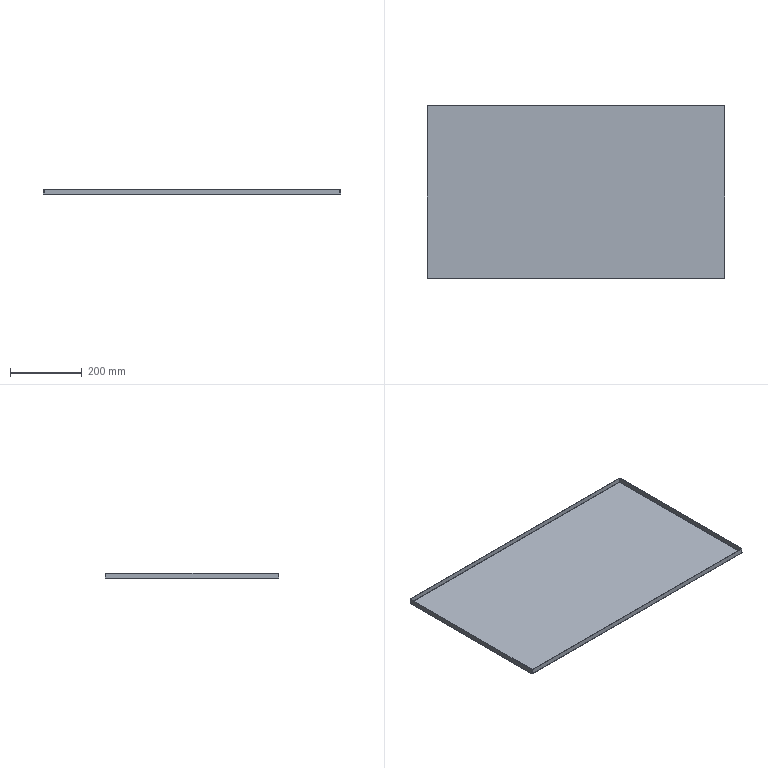Part | SolidWorks | 1 solid | 38 faces | box 830.001 x 485.001 x 15 mm | volume 655273 mm3 | plane 22 | spline 8 | cylinder 8 | commonest cylinder face diameters 0.2 x4 3.2 x4
STEP:
#1=CARTESIAN_POINT('',(413.4,-240.9,-1.5));
#2=VERTEX_POINT('',#1);
#3=CARTESIAN_POINT('',(-413.4,-240.9,-1.5));
#4=VERTEX_POINT('',#3);
#5=CARTESIAN_POINT('',(413.4,-240.9,-1.5));
#6=DIRECTION('',(-1.,0.,0.));
#7=VECTOR('',#6,1000.);
#8=LINE('',#5,#7);
#9=EDGE_CURVE('',#2,#4,#8,.T.);
#10=ORIENTED_EDGE('',*,*,#9,.T.);
#11=CARTESIAN_POINT('',(-413.4,240.9,-1.5));
#12=VERTEX_POINT('',#11);
#13=CARTESIAN_POINT('',(-413.4,-240.9,-1.5));
#14=DIRECTION('',(0.,1.,0.));
#15=VECTOR('',#14,1000.);
#16=LINE('',#13,#15);
#17=EDGE_CURVE('',#4,#12,#16,.T.);
#18=ORIENTED_EDGE('',*,*,#17,.T.);
#19=CARTESIAN_POINT('',(413.4,240.9,-1.5));
#20=VERTEX_POINT('',#19);
#21=CARTESIAN_POINT('',(-413.4,240.9,-1.5));
#22=DIRECTION('',(1.,0.,0.));
#23=VECTOR('',#22,1000.);
#24=LINE('',#21,#23);
#25=EDGE_CURVE('',#12,#20,#24,.T.);
#26=ORIENTED_EDGE('',*,*,#25,.T.);
#27=CARTESIAN_POINT('',(413.4,240.9,-1.5));
#28=DIRECTION('',(0.,-1.,0.));
#29=VECTOR('',#28,1000.);
#30=LINE('',#27,#29);
#31=EDGE_CURVE('',#20,#2,#30,.T.);
#32=ORIENTED_EDGE('',*,*,#31,.T.);
#33=EDGE_LOOP('',(#10,#18,#26,#32));
#34=FACE_OUTER_BOUND('',#33,.T.);
#35=CARTESIAN_POINT('',(0.,0.,-1.5));
#36=DIRECTION('',(0.,0.,1.));
#37=DIRECTION('',(1.,0.,0.));
#38=AXIS2_PLACEMENT_3D('',#35,#36,#37);
#39=PLANE('',#38);
#40=ADVANCED_FACE('',(#34),#39,.F.);
#41=CARTESIAN_POINT('',(-413.4,-240.9,0.));
#42=VERTEX_POINT('',#41);
#43=CARTESIAN_POINT('',(-413.4,240.9,0.));
#44=VERTEX_POINT('',#43);
#45=CARTESIAN_POINT('',(-413.4,-240.9,0.));
#46=DIRECTION('',(0.,1.,0.));
#47=VECTOR('',#46,1000.);
#48=LINE('',#45,#47);
#49=EDGE_CURVE('',#42,#44,#48,.T.);
#50=ORIENTED_EDGE('',*,*,#49,.F.);
#51=CARTESIAN_POINT('',(413.4,-240.9,0.));
#52=VERTEX_POINT('',#51);
#53=CARTESIAN_POINT('',(413.4,-240.9,0.));
#54=DIRECTION('',(-1.,0.,0.));
#55=VECTOR('',#54,1000.);
#56=LINE('',#53,#55);
#57=EDGE_CURVE('',#52,#42,#56,.T.);
#58=ORIENTED_EDGE('',*,*,#57,.F.);
#59=CARTESIAN_POINT('',(413.4,240.9,0.));
#60=VERTEX_POINT('',#59);
#61=CARTESIAN_POINT('',(413.4,240.9,0.));
#62=DIRECTION('',(0.,-1.,0.));
#63=VECTOR('',#62,1000.);
#64=LINE('',#61,#63);
#65=EDGE_CURVE('',#60,#52,#64,.T.);
#66=ORIENTED_EDGE('',*,*,#65,.F.);
#67=CARTESIAN_POINT('',(-413.4,240.9,0.));
#68=DIRECTION('',(1.,0.,0.));
#69=VECTOR('',#68,1000.);
#70=LINE('',#67,#69);
#71=EDGE_CURVE('',#44,#60,#70,.T.);
#72=ORIENTED_EDGE('',*,*,#71,.F.);
#73=EDGE_LOOP('',(#50,#58,#66,#72));
#74=FACE_OUTER_BOUND('',#73,.T.);
#75=CARTESIAN_POINT('',(0.,0.,0.));
#76=DIRECTION('',(0.,0.,1.));
#77=DIRECTION('',(1.,0.,0.));
#78=AXIS2_PLACEMENT_3D('',#75,#76,#77);
#79=PLANE('',#78);
#80=ADVANCED_FACE('',(#74),#79,.T.);
#81=CARTESIAN_POINT('',(-415.,240.293,0.1));
#82=VERTEX_POINT('',#81);
#83=CARTESIAN_POINT('',(-413.5,240.293,0.1));
#84=VERTEX_POINT('',#83);
#85=CARTESIAN_POINT('',(-413.5,240.293,0.1));
#86=DIRECTION('',(1.,0.,0.));
#87=VECTOR('',#86,1000.);
#88=LINE('',#85,#87);
#89=EDGE_CURVE('',#82,#84,#88,.T.);
#90=ORIENTED_EDGE('',*,*,#89,.T.);
#91=CARTESIAN_POINT('',(-413.4,240.9,0.));
#92=CARTESIAN_POINT('',(-413.426,240.799,0.));
#93=CARTESIAN_POINT('',(-413.452,240.698,0.01078));
#94=CARTESIAN_POINT('',(-413.489,240.495,0.0478));
#95=CARTESIAN_POINT('',(-413.5,240.394,0.07382));
#96=CARTESIAN_POINT('',(-413.5,240.293,0.1));
#97=B_SPLINE_CURVE_WITH_KNOTS('',3,(#91,#92,#93,#94,#95,#96),.UNSPECIFIED.,.F.,.F.,(4,2,4),(0.,0.5,1.),.UNSPECIFIED.);
#98=EDGE_CURVE('',#44,#84,#97,.T.);
#99=ORIENTED_EDGE('',*,*,#98,.F.);
#100=CARTESIAN_POINT('',(-413.4,240.9,0.));
#101=DIRECTION('',(0.,0.,-1.));
#102=VECTOR('',#101,1000.);
#103=LINE('',#100,#102);
#104=EDGE_CURVE('',#44,#12,#103,.T.);
#105=ORIENTED_EDGE('',*,*,#104,.T.);
#106=CARTESIAN_POINT('',(-413.4,240.9,-1.5));
#107=CARTESIAN_POINT('',(-413.612,240.849,-1.5));
#108=CARTESIAN_POINT('',(-413.815,240.8,-1.46));
#109=CARTESIAN_POINT('',(-414.205,240.698,-1.299));
#110=CARTESIAN_POINT('',(-414.381,240.648,-1.181));
#111=CARTESIAN_POINT('',(-414.605,240.571,-0.9582));
#112=CARTESIAN_POINT('',(-414.671,240.546,-0.8775));
#113=CARTESIAN_POINT('',(-414.787,240.496,-0.7041));
#114=CARTESIAN_POINT('',(-414.838,240.47,-0.6103));
#115=CARTESIAN_POINT('',(-414.958,240.394,-0.32));
#116=CARTESIAN_POINT('',(-415.,240.344,-0.1115));
#117=CARTESIAN_POINT('',(-415.,240.293,0.1));
#118=B_SPLINE_CURVE_WITH_KNOTS('',3,(#106,#107,#108,#109,#110,#111,#112,#113,#114,#115,#116,#117),.UNSPECIFIED.,.F.,.F.,(4,2,2,2,2,4),(0.,0.0006399,0.00128,0.0016,0.00192,0.00256),.UNSPECIFIED.);
#119=EDGE_CURVE('',#12,#82,#118,.T.);
#120=ORIENTED_EDGE('',*,*,#119,.T.);
#121=EDGE_LOOP('',(#90,#99,#105,#120));
#122=FACE_OUTER_BOUND('',#121,.T.);
#123=CARTESIAN_POINT('',(-413.4,240.9,-1.515));
#124=CARTESIAN_POINT('',(-413.611,240.849,-1.515));
#125=CARTESIAN_POINT('',(-413.823,240.799,-1.473));
#126=CARTESIAN_POINT('',(-414.213,240.698,-1.311));
#127=CARTESIAN_POINT('',(-414.392,240.647,-1.191));
#128=CARTESIAN_POINT('',(-414.691,240.546,-0.8925));
#129=CARTESIAN_POINT('',(-414.811,240.495,-0.7133));
#130=CARTESIAN_POINT('',(-414.973,240.394,-0.3227));
#131=CARTESIAN_POINT('',(-415.015,240.343,-0.1114));
#132=CARTESIAN_POINT('',(-415.015,240.293,0.1));
#133=CARTESIAN_POINT('',(-413.4,240.9,-1.5));
#134=CARTESIAN_POINT('',(-413.609,240.849,-1.5));
#135=CARTESIAN_POINT('',(-413.819,240.799,-1.458));
#136=CARTESIAN_POINT('',(-414.206,240.698,-1.298));
#137=CARTESIAN_POINT('',(-414.383,240.647,-1.179));
#138=CARTESIAN_POINT('',(-414.679,240.546,-0.8833));
#139=CARTESIAN_POINT('',(-414.798,240.495,-0.7058));
#140=CARTESIAN_POINT('',(-414.958,240.394,-0.3188));
#141=CARTESIAN_POINT('',(-415.,240.343,-0.1095));
#142=CARTESIAN_POINT('',(-415.,240.293,0.1));
#143=CARTESIAN_POINT('',(-413.4,240.9,0.));
#144=CARTESIAN_POINT('',(-413.413,240.849,0.));
#145=CARTESIAN_POINT('',(-413.426,240.799,0.002603));
#146=CARTESIAN_POINT('',(-413.45,240.698,0.01262));
#147=CARTESIAN_POINT('',(-413.461,240.647,0.02003));
#148=CARTESIAN_POINT('',(-413.48,240.546,0.03855));
#149=CARTESIAN_POINT('',(-413.487,240.495,0.04964));
#150=CARTESIAN_POINT('',(-413.497,240.394,0.07383));
#151=CARTESIAN_POINT('',(-413.5,240.343,0.08691));
#152=CARTESIAN_POINT('',(-413.5,240.293,0.1));
#153=B_SPLINE_SURFACE_WITH_KNOTS('',1,3,((#123,#124,#125,#126,#127,#128,#129,#130,#131,#132),(#133,#134,#135,#136,#137,#138,#139,#140,#141,#142),(#143,#144,#145,#146,#147,#148,#149,#150,#151,#152)),.UNSPECIFIED.,.F.,.F.,.F.,(2,1,2),(4,2,2,2,4),(-0.01,0.,1.),(0.,0.25,0.5,0.75,1.),.UNSPECIFIED.);
#154=ADVANCED_FACE('',(#122),#153,.F.);
#155=CARTESIAN_POINT('',(-413.5,-240.293,0.1));
#156=VERTEX_POINT('',#155);
#157=CARTESIAN_POINT('',(-413.5,-240.293,0.1));
#158=CARTESIAN_POINT('',(-413.5,-240.394,0.07382));
#159=CARTESIAN_POINT('',(-413.489,-240.495,0.0478));
#160=CARTESIAN_POINT('',(-413.452,-240.698,0.01078));
#161=CARTESIAN_POINT('',(-413.426,-240.799,0.));
#162=CARTESIAN_POINT('',(-413.4,-240.9,0.));
#163=B_SPLINE_CURVE_WITH_KNOTS('',3,(#157,#158,#159,#160,#161,#162),.UNSPECIFIED.,.F.,.F.,(4,2,4),(0.,0.5,1.),.UNSPECIFIED.);
#164=EDGE_CURVE('',#156,#42,#163,.T.);
#165=ORIENTED_EDGE('',*,*,#164,.F.);
#166=CARTESIAN_POINT('',(-415.,-240.293,0.1));
#167=VERTEX_POINT('',#166);
#168=CARTESIAN_POINT('',(-413.5,-240.293,0.1));
#169=DIRECTION('',(1.,0.,0.));
#170=VECTOR('',#169,1000.);
#171=LINE('',#168,#170);
#172=EDGE_CURVE('',#167,#156,#171,.T.);
#173=ORIENTED_EDGE('',*,*,#172,.F.);
#174=CARTESIAN_POINT('',(-415.,-240.293,0.1));
#175=CARTESIAN_POINT('',(-415.,-240.344,-0.1115));
#176=CARTESIAN_POINT('',(-414.96,-240.393,-0.3151));
#177=CARTESIAN_POINT('',(-414.799,-240.495,-0.7048));
#178=CARTESIAN_POINT('',(-414.681,-240.545,-0.881));
#179=CARTESIAN_POINT('',(-414.458,-240.621,-1.105));
#180=CARTESIAN_POINT('',(-414.378,-240.647,-1.171));
#181=CARTESIAN_POINT('',(-414.204,-240.697,-1.287));
#182=CARTESIAN_POINT('',(-414.11,-240.723,-1.338));
#183=CARTESIAN_POINT('',(-413.82,-240.799,-1.458));
#184=CARTESIAN_POINT('',(-413.612,-240.849,-1.5));
#185=CARTESIAN_POINT('',(-413.4,-240.9,-1.5));
#186=B_SPLINE_CURVE_WITH_KNOTS('',3,(#174,#175,#176,#177,#178,#179,#180,#181,#182,#183,#184,#185),.UNSPECIFIED.,.F.,.F.,(4,2,2,2,2,4),(0.,0.0006399,0.00128,0.0016,0.00192,0.00256),.UNSPECIFIED.);
#187=EDGE_CURVE('',#167,#4,#186,.T.);
#188=ORIENTED_EDGE('',*,*,#187,.T.);
#189=CARTESIAN_POINT('',(-413.4,-240.9,0.));
#190=DIRECTION('',(0.,0.,-1.));
#191=VECTOR('',#190,1000.);
#192=LINE('',#189,#191);
#193=EDGE_CURVE('',#42,#4,#192,.T.);
#194=ORIENTED_EDGE('',*,*,#193,.F.);
#195=EDGE_LOOP('',(#165,#173,#188,#194));
#196=FACE_OUTER_BOUND('',#195,.T.);
#197=CARTESIAN_POINT('',(-415.015,-240.293,0.1));
#198=CARTESIAN_POINT('',(-415.015,-240.343,-0.1114));
#199=CARTESIAN_POINT('',(-414.973,-240.394,-0.3227));
#200=CARTESIAN_POINT('',(-414.811,-240.495,-0.7133));
#201=CARTESIAN_POINT('',(-414.691,-240.546,-0.8925));
#202=CARTESIAN_POINT('',(-414.392,-240.647,-1.191));
#203=CARTESIAN_POINT('',(-414.213,-240.698,-1.311));
#204=CARTESIAN_POINT('',(-413.823,-240.799,-1.473));
#205=CARTESIAN_POINT('',(-413.611,-240.849,-1.515));
#206=CARTESIAN_POINT('',(-413.4,-240.9,-1.515));
#207=CARTESIAN_POINT('',(-415.,-240.293,0.1));
#208=CARTESIAN_POINT('',(-415.,-240.343,-0.1095));
#209=CARTESIAN_POINT('',(-414.958,-240.394,-0.3188));
#210=CARTESIAN_POINT('',(-414.798,-240.495,-0.7058));
#211=CARTESIAN_POINT('',(-414.679,-240.546,-0.8833));
#212=CARTESIAN_POINT('',(-414.383,-240.647,-1.179));
#213=CARTESIAN_POINT('',(-414.206,-240.698,-1.298));
#214=CARTESIAN_POINT('',(-413.819,-240.799,-1.458));
#215=CARTESIAN_POINT('',(-413.609,-240.849,-1.5));
#216=CARTESIAN_POINT('',(-413.4,-240.9,-1.5));
#217=CARTESIAN_POINT('',(-413.5,-240.293,0.1));
#218=CARTESIAN_POINT('',(-413.5,-240.343,0.08691));
#219=CARTESIAN_POINT('',(-413.497,-240.394,0.07383));
#220=CARTESIAN_POINT('',(-413.487,-240.495,0.04964));
#221=CARTESIAN_POINT('',(-413.48,-240.546,0.03855));
#222=CARTESIAN_POINT('',(-413.461,-240.647,0.02003));
#223=CARTESIAN_POINT('',(-413.45,-240.698,0.01262));
#224=CARTESIAN_POINT('',(-413.426,-240.799,0.002603));
#225=CARTESIAN_POINT('',(-413.413,-240.849,0.));
#226=CARTESIAN_POINT('',(-413.4,-240.9,0.));
#227=B_SPLINE_SURFACE_WITH_KNOTS('',1,3,((#197,#198,#199,#200,#201,#202,#203,#204,#205,#206),(#207,#208,#209,#210,#211,#212,#213,#214,#215,#216),(#217,#218,#219,#220,#221,#222,#223,#224,#225,#226)),.UNSPECIFIED.,.F.,.F.,.F.,(2,1,2),(4,2,2,2,4),(-0.01,0.,1.),(0.,0.25,0.5,0.75,1.),.UNSPECIFIED.);
#228=ADVANCED_FACE('',(#196),#227,.F.);
#229=ORIENTED_EDGE('',*,*,#17,.F.);
#230=ORIENTED_EDGE('',*,*,#187,.F.);
#231=CARTESIAN_POINT('',(-415.,242.5,0.1));
#232=DIRECTION('',(0.,1.,0.));
#233=VECTOR('',#232,1000.);
#234=LINE('',#231,#233);
#235=EDGE_CURVE('',#167,#82,#234,.T.);
#236=ORIENTED_EDGE('',*,*,#235,.T.);
#237=ORIENTED_EDGE('',*,*,#119,.F.);
#238=EDGE_LOOP('',(#229,#230,#236,#237));
#239=FACE_OUTER_BOUND('',#238,.T.);
#240=CARTESIAN_POINT('',(-413.4,-240.9,0.1));
#241=DIRECTION('',(0.,-1.,0.));
#242=DIRECTION('',(-1.,0.,0.));
#243=AXIS2_PLACEMENT_3D('',#240,#241,#242);
#244=CYLINDRICAL_SURFACE('',#243,1.6);
#245=ADVANCED_FACE('',(#239),#244,.T.);
#246=ORIENTED_EDGE('',*,*,#49,.T.);
#247=ORIENTED_EDGE('',*,*,#98,.T.);
#248=CARTESIAN_POINT('',(-413.5,242.5,0.1));
#249=DIRECTION('',(0.,-1.,0.));
#250=VECTOR('',#249,1000.);
#251=LINE('',#248,#250);
#252=EDGE_CURVE('',#84,#156,#251,.T.);
#253=ORIENTED_EDGE('',*,*,#252,.T.);
#254=ORIENTED_EDGE('',*,*,#164,.T.);
#255=EDGE_LOOP('',(#246,#247,#253,#254));
#256=FACE_OUTER_BOUND('',#255,.T.);
#257=CARTESIAN_POINT('',(-413.4,-240.9,0.1));
#258=DIRECTION('',(0.,-1.,0.));
#259=DIRECTION('',(-1.,0.,0.));
#260=AXIS2_PLACEMENT_3D('',#257,#258,#259);
#261=CYLINDRICAL_SURFACE('',#260,0.1);
#262=ADVANCED_FACE('',(#256),#261,.F.);
#263=CARTESIAN_POINT('',(-415.,240.293,13.5));
#264=VERTEX_POINT('',#263);
#265=CARTESIAN_POINT('',(-415.,240.293,0.));
#266=DIRECTION('',(0.,0.,1.));
#267=VECTOR('',#266,1000.);
#268=LINE('',#265,#267);
#269=EDGE_CURVE('',#82,#264,#268,.T.);
#270=ORIENTED_EDGE('',*,*,#269,.T.);
#271=CARTESIAN_POINT('',(-413.5,240.293,13.5));
#272=VERTEX_POINT('',#271);
#273=CARTESIAN_POINT('',(-413.5,240.293,13.5));
#274=DIRECTION('',(1.,0.,0.));
#275=VECTOR('',#274,1000.);
#276=LINE('',#273,#275);
#277=EDGE_CURVE('',#264,#272,#276,.T.);
#278=ORIENTED_EDGE('',*,*,#277,.T.);
#279=CARTESIAN_POINT('',(-413.5,240.293,0.));
#280=DIRECTION('',(0.,0.,1.));
#281=VECTOR('',#280,1000.);
#282=LINE('',#279,#281);
#283=EDGE_CURVE('',#84,#272,#282,.T.);
#284=ORIENTED_EDGE('',*,*,#283,.F.);
#285=ORIENTED_EDGE('',*,*,#89,.F.);
#286=EDGE_LOOP('',(#270,#278,#284,#285));
#287=FACE_OUTER_BOUND('',#286,.T.);
#288=CARTESIAN_POINT('',(-413.5,240.293,0.));
#289=DIRECTION('',(0.,1.,0.));
#290=DIRECTION('',(0.,0.,1.));
#291=AXIS2_PLACEMENT_3D('',#288,#289,#290);
#292=PLANE('',#291);
#293=ADVANCED_FACE('',(#287),#292,.T.);
#294=ORIENTED_EDGE('',*,*,#235,.F.);
#295=CARTESIAN_POINT('',(-415.,-240.293,13.5));
#296=VERTEX_POINT('',#295);
#297=CARTESIAN_POINT('',(-415.,-240.293,0.));
#298=DIRECTION('',(0.,0.,1.));
#299=VECTOR('',#298,1000.);
#300=LINE('',#297,#299);
#301=EDGE_CURVE('',#167,#296,#300,.T.);
#302=ORIENTED_EDGE('',*,*,#301,.T.);
#303=CARTESIAN_POINT('',(-415.,0.,13.5));
#304=DIRECTION('',(0.,1.,0.));
#305=VECTOR('',#304,1000.);
#306=LINE('',#303,#305);
#307=EDGE_CURVE('',#296,#264,#306,.T.);
#308=ORIENTED_EDGE('',*,*,#307,.T.);
#309=ORIENTED_EDGE('',*,*,#269,.F.);
#310=EDGE_LOOP('',(#294,#302,#308,#309));
#311=FACE_OUTER_BOUND('',#310,.T.);
#312=CARTESIAN_POINT('',(-415.,0.,0.));
#313=DIRECTION('',(1.,0.,0.));
#314=DIRECTION('',(0.,0.,-1.));
#315=AXIS2_PLACEMENT_3D('',#312,#313,#314);
#316=PLANE('',#315);
#317=ADVANCED_FACE('',(#311),#316,.F.);
#318=CARTESIAN_POINT('',(-413.5,-240.293,13.5));
#319=VERTEX_POINT('',#318);
#320=CARTESIAN_POINT('',(-413.5,-240.293,0.));
#321=DIRECTION('',(0.,0.,1.));
#322=VECTOR('',#321,1000.);
#323=LINE('',#320,#322);
#324=EDGE_CURVE('',#156,#319,#323,.T.);
#325=ORIENTED_EDGE('',*,*,#324,.F.);
#326=ORIENTED_EDGE('',*,*,#252,.F.);
#327=ORIENTED_EDGE('',*,*,#283,.T.);
#328=CARTESIAN_POINT('',(-413.5,242.5,13.5));
#329=DIRECTION('',(0.,1.,0.));
#330=VECTOR('',#329,1000.);
#331=LINE('',#328,#330);
#332=EDGE_CURVE('',#319,#272,#331,.T.);
#333=ORIENTED_EDGE('',*,*,#332,.F.);
#334=EDGE_LOOP('',(#325,#326,#327,#333));
#335=FACE_OUTER_BOUND('',#334,.T.);
#336=CARTESIAN_POINT('',(-413.5,0.,0.));
#337=DIRECTION('',(1.,0.,0.));
#338=DIRECTION('',(0.,0.,-1.));
#339=AXIS2_PLACEMENT_3D('',#336,#337,#338);
#340=PLANE('',#339);
#341=ADVANCED_FACE('',(#335),#340,.T.);
#342=ORIENTED_EDGE('',*,*,#307,.F.);
#343=CARTESIAN_POINT('',(-415.,-240.293,13.5));
#344=DIRECTION('',(1.,0.,0.));
#345=VECTOR('',#344,1000.);
#346=LINE('',#343,#345);
#347=EDGE_CURVE('',#296,#319,#346,.T.);
#348=ORIENTED_EDGE('',*,*,#347,.T.);
#349=ORIENTED_EDGE('',*,*,#332,.T.);
#350=ORIENTED_EDGE('',*,*,#277,.F.);
#351=EDGE_LOOP('',(#342,#348,#349,#350));
#352=FACE_OUTER_BOUND('',#351,.T.);
#353=CARTESIAN_POINT('',(-415.,242.5,13.5));
#354=DIRECTION('',(0.,0.,-1.));
#355=DIRECTION('',(-1.,0.,0.));
#356=AXIS2_PLACEMENT_3D('',#353,#354,#355);
#357=PLANE('',#356);
#358=ADVANCED_FACE('',(#352),#357,.F.);
#359=ORIENTED_EDGE('',*,*,#347,.F.);
#360=ORIENTED_EDGE('',*,*,#301,.F.);
#361=ORIENTED_EDGE('',*,*,#172,.T.);
#362=ORIENTED_EDGE('',*,*,#324,.T.);
#363=EDGE_LOOP('',(#359,#360,#361,#362));
#364=FACE_OUTER_BOUND('',#363,.T.);
#365=CARTESIAN_POINT('',(-413.5,-240.293,0.));
#366=DIRECTION('',(0.,1.,0.));
#367=DIRECTION('',(0.,0.,1.));
#368=AXIS2_PLACEMENT_3D('',#365,#366,#367);
#369=PLANE('',#368);
#370=ADVANCED_FACE('',(#364),#369,.F.);
#371=CARTESIAN_POINT('',(412.793,242.5,0.1));
#372=VERTEX_POINT('',#371);
#373=CARTESIAN_POINT('',(412.793,241.,0.1));
#374=VERTEX_POINT('',#373);
#375=CARTESIAN_POINT('',(412.793,241.,0.1));
#376=DIRECTION('',(0.,-1.,0.));
#377=VECTOR('',#376,1000.);
#378=LINE('',#375,#377);
#379=EDGE_CURVE('',#372,#374,#378,.T.);
#380=ORIENTED_EDGE('',*,*,#379,.T.);
#381=CARTESIAN_POINT('',(413.4,240.9,0.));
#382=CARTESIAN_POINT('',(413.299,240.926,0.));
#383=CARTESIAN_POINT('',(413.198,240.952,0.01078));
#384=CARTESIAN_POINT('',(412.995,240.989,0.0478));
#385=CARTESIAN_POINT('',(412.894,241.,0.07382));
#386=CARTESIAN_POINT('',(412.793,241.,0.1));
#387=B_SPLINE_CURVE_WITH_KNOTS('',3,(#381,#382,#383,#384,#385,#386),.UNSPECIFIED.,.F.,.F.,(4,2,4),(0.,0.5,1.),.UNSPECIFIED.);
#388=EDGE_CURVE('',#60,#374,#387,.T.);
#389=ORIENTED_EDGE('',*,*,#388,.F.);
#390=CARTESIAN_POINT('',(413.4,240.9,0.));
#391=DIRECTION('',(0.,0.,-1.));
#392=VECTOR('',#391,1000.);
#393=LINE('',#390,#392);
#394=EDGE_CURVE('',#60,#20,#393,.T.);
#395=ORIENTED_EDGE('',*,*,#394,.T.);
#396=CARTESIAN_POINT('',(413.4,240.9,-1.5));
#397=CARTESIAN_POINT('',(413.349,241.112,-1.5));
#398=CARTESIAN_POINT('',(413.3,241.315,-1.46));
#399=CARTESIAN_POINT('',(413.198,241.705,-1.299));
#400=CARTESIAN_POINT('',(413.148,241.881,-1.181));
#401=CARTESIAN_POINT('',(413.071,242.105,-0.9582));
#402=CARTESIAN_POINT('',(413.046,242.171,-0.8775));
#403=CARTESIAN_POINT('',(412.996,242.287,-0.7041));
#404=CARTESIAN_POINT('',(412.97,242.338,-0.6103));
#405=CARTESIAN_POINT('',(412.894,242.458,-0.32));
#406=CARTESIAN_POINT('',(412.844,242.5,-0.1115));
#407=CARTESIAN_POINT('',(412.793,242.5,0.1));
#408=B_SPLINE_CURVE_WITH_KNOTS('',3,(#396,#397,#398,#399,#400,#401,#402,#403,#404,#405,#406,#407),.UNSPECIFIED.,.F.,.F.,(4,2,2,2,2,4),(0.,0.0006399,0.00128,0.0016,0.00192,0.00256),.UNSPECIFIED.);
#409=EDGE_CURVE('',#20,#372,#408,.T.);
#410=ORIENTED_EDGE('',*,*,#409,.T.);
#411=EDGE_LOOP('',(#380,#389,#395,#410));
#412=FACE_OUTER_BOUND('',#411,.T.);
#413=CARTESIAN_POINT('',(413.4,240.9,-1.515));
#414=CARTESIAN_POINT('',(413.349,241.111,-1.515));
#415=CARTESIAN_POINT('',(413.299,241.323,-1.473));
#416=CARTESIAN_POINT('',(413.198,241.713,-1.311));
#417=CARTESIAN_POINT('',(413.147,241.892,-1.191));
#418=CARTESIAN_POINT('',(413.046,242.191,-0.8925));
#419=CARTESIAN_POINT('',(412.995,242.311,-0.7133));
#420=CARTESIAN_POINT('',(412.894,242.473,-0.3227));
#421=CARTESIAN_POINT('',(412.843,242.515,-0.1114));
#422=CARTESIAN_POINT('',(412.793,242.515,0.1));
#423=CARTESIAN_POINT('',(413.4,240.9,-1.5));
#424=CARTESIAN_POINT('',(413.349,241.109,-1.5));
#425=CARTESIAN_POINT('',(413.299,241.319,-1.458));
#426=CARTESIAN_POINT('',(413.198,241.706,-1.298));
#427=CARTESIAN_POINT('',(413.147,241.883,-1.179));
#428=CARTESIAN_POINT('',(413.046,242.179,-0.8833));
#429=CARTESIAN_POINT('',(412.995,242.298,-0.7058));
#430=CARTESIAN_POINT('',(412.894,242.458,-0.3188));
#431=CARTESIAN_POINT('',(412.843,242.5,-0.1095));
#432=CARTESIAN_POINT('',(412.793,242.5,0.1));
#433=CARTESIAN_POINT('',(413.4,240.9,0.));
#434=CARTESIAN_POINT('',(413.349,240.913,0.));
#435=CARTESIAN_POINT('',(413.299,240.926,0.002603));
#436=CARTESIAN_POINT('',(413.198,240.95,0.01262));
#437=CARTESIAN_POINT('',(413.147,240.961,0.02003));
#438=CARTESIAN_POINT('',(413.046,240.98,0.03855));
#439=CARTESIAN_POINT('',(412.995,240.987,0.04964));
#440=CARTESIAN_POINT('',(412.894,240.997,0.07383));
#441=CARTESIAN_POINT('',(412.843,241.,0.08691));
#442=CARTESIAN_POINT('',(412.793,241.,0.1));
#443=B_SPLINE_SURFACE_WITH_KNOTS('',1,3,((#413,#414,#415,#416,#417,#418,#419,#420,#421,#422),(#423,#424,#425,#426,#427,#428,#429,#430,#431,#432),(#433,#434,#435,#436,#437,#438,#439,#440,#441,#442)),.UNSPECIFIED.,.F.,.F.,.F.,(2,1,2),(4,2,2,2,4),(-0.01,0.,1.),(0.,0.25,0.5,0.75,1.),.UNSPECIFIED.);
#444=ADVANCED_FACE('',(#412),#443,.F.);
#445=CARTESIAN_POINT('',(-412.793,241.,0.1));
#446=VERTEX_POINT('',#445);
#447=CARTESIAN_POINT('',(-412.793,241.,0.1));
#448=CARTESIAN_POINT('',(-412.894,241.,0.07382));
#449=CARTESIAN_POINT('',(-412.995,240.989,0.0478));
#450=CARTESIAN_POINT('',(-413.198,240.952,0.01078));
#451=CARTESIAN_POINT('',(-413.299,240.926,0.));
#452=CARTESIAN_POINT('',(-413.4,240.9,0.));
#453=B_SPLINE_CURVE_WITH_KNOTS('',3,(#447,#448,#449,#450,#451,#452),.UNSPECIFIED.,.F.,.F.,(4,2,4),(0.,0.5,1.),.UNSPECIFIED.);
#454=EDGE_CURVE('',#446,#44,#453,.T.);
#455=ORIENTED_EDGE('',*,*,#454,.F.);
#456=CARTESIAN_POINT('',(-412.793,242.5,0.1));
#457=VERTEX_POINT('',#456);
#458=CARTESIAN_POINT('',(-412.793,241.,0.1));
#459=DIRECTION('',(0.,-1.,0.));
#460=VECTOR('',#459,1000.);
#461=LINE('',#458,#460);
#462=EDGE_CURVE('',#457,#446,#461,.T.);
#463=ORIENTED_EDGE('',*,*,#462,.F.);
#464=CARTESIAN_POINT('',(-412.793,242.5,0.1));
#465=CARTESIAN_POINT('',(-412.844,242.5,-0.1115));
#466=CARTESIAN_POINT('',(-412.893,242.46,-0.3151));
#467=CARTESIAN_POINT('',(-412.995,242.299,-0.7048));
#468=CARTESIAN_POINT('',(-413.045,242.181,-0.881));
#469=CARTESIAN_POINT('',(-413.121,241.958,-1.105));
#470=CARTESIAN_POINT('',(-413.147,241.878,-1.171));
#471=CARTESIAN_POINT('',(-413.197,241.704,-1.287));
#472=CARTESIAN_POINT('',(-413.223,241.61,-1.338));
#473=CARTESIAN_POINT('',(-413.299,241.32,-1.458));
#474=CARTESIAN_POINT('',(-413.349,241.112,-1.5));
#475=CARTESIAN_POINT('',(-413.4,240.9,-1.5));
#476=B_SPLINE_CURVE_WITH_KNOTS('',3,(#464,#465,#466,#467,#468,#469,#470,#471,#472,#473,#474,#475),.UNSPECIFIED.,.F.,.F.,(4,2,2,2,2,4),(0.,0.0006399,0.00128,0.0016,0.00192,0.00256),.UNSPECIFIED.);
#477=EDGE_CURVE('',#457,#12,#476,.T.);
#478=ORIENTED_EDGE('',*,*,#477,.T.);
#479=ORIENTED_EDGE('',*,*,#104,.F.);
#480=EDGE_LOOP('',(#455,#463,#478,#479));
#481=FACE_OUTER_BOUND('',#480,.T.);
#482=CARTESIAN_POINT('',(-412.793,242.515,0.1));
#483=CARTESIAN_POINT('',(-412.843,242.515,-0.1114));
#484=CARTESIAN_POINT('',(-412.894,242.473,-0.3227));
#485=CARTESIAN_POINT('',(-412.995,242.311,-0.7133));
#486=CARTESIAN_POINT('',(-413.046,242.191,-0.8925));
#487=CARTESIAN_POINT('',(-413.147,241.892,-1.191));
#488=CARTESIAN_POINT('',(-413.198,241.713,-1.311));
#489=CARTESIAN_POINT('',(-413.299,241.323,-1.473));
#490=CARTESIAN_POINT('',(-413.349,241.111,-1.515));
#491=CARTESIAN_POINT('',(-413.4,240.9,-1.515));
#492=CARTESIAN_POINT('',(-412.793,242.5,0.1));
#493=CARTESIAN_POINT('',(-412.843,242.5,-0.1095));
#494=CARTESIAN_POINT('',(-412.894,242.458,-0.3188));
#495=CARTESIAN_POINT('',(-412.995,242.298,-0.7058));
#496=CARTESIAN_POINT('',(-413.046,242.179,-0.8833));
#497=CARTESIAN_POINT('',(-413.147,241.883,-1.179));
#498=CARTESIAN_POINT('',(-413.198,241.706,-1.298));
#499=CARTESIAN_POINT('',(-413.299,241.319,-1.458));
#500=CARTESIAN_POINT('',(-413.349,241.109,-1.5));
#501=CARTESIAN_POINT('',(-413.4,240.9,-1.5));
#502=CARTESIAN_POINT('',(-412.793,241.,0.1));
#503=CARTESIAN_POINT('',(-412.843,241.,0.08691));
#504=CARTESIAN_POINT('',(-412.894,240.997,0.07383));
#505=CARTESIAN_POINT('',(-412.995,240.987,0.04964));
#506=CARTESIAN_POINT('',(-413.046,240.98,0.03855));
#507=CARTESIAN_POINT('',(-413.147,240.961,0.02003));
#508=CARTESIAN_POINT('',(-413.198,240.95,0.01262));
#509=CARTESIAN_POINT('',(-413.299,240.926,0.002603));
#510=CARTESIAN_POINT('',(-413.349,240.913,0.));
#511=CARTESIAN_POINT('',(-413.4,240.9,0.));
#512=B_SPLINE_SURFACE_WITH_KNOTS('',1,3,((#482,#483,#484,#485,#486,#487,#488,#489,#490,#491),(#492,#493,#494,#495,#496,#497,#498,#499,#500,#501),(#502,#503,#504,#505,#506,#507,#508,#509,#510,#511)),.UNSPECIFIED.,.F.,.F.,.F.,(2,1,2),(4,2,2,2,4),(-0.01,0.,1.),(0.,0.25,0.5,0.75,1.),.UNSPECIFIED.);
#513=ADVANCED_FACE('',(#481),#512,.F.);
#514=ORIENTED_EDGE('',*,*,#25,.F.);
#515=ORIENTED_EDGE('',*,*,#477,.F.);
#516=CARTESIAN_POINT('',(415.,242.5,0.1));
#517=DIRECTION('',(1.,0.,0.));
#518=VECTOR('',#517,1000.);
#519=LINE('',#516,#518);
#520=EDGE_CURVE('',#457,#372,#519,.T.);
#521=ORIENTED_EDGE('',*,*,#520,.T.);
#522=ORIENTED_EDGE('',*,*,#409,.F.);
#523=EDGE_LOOP('',(#514,#515,#521,#522));
#524=FACE_OUTER_BOUND('',#523,.T.);
#525=CARTESIAN_POINT('',(-413.4,240.9,0.1));
#526=DIRECTION('',(-1.,0.,0.));
#527=DIRECTION('',(0.,1.,0.));
#528=AXIS2_PLACEMENT_3D('',#525,#526,#527);
#529=CYLINDRICAL_SURFACE('',#528,1.6);
#530=ADVANCED_FACE('',(#524),#529,.T.);
#531=ORIENTED_EDGE('',*,*,#71,.T.);
#532=ORIENTED_EDGE('',*,*,#388,.T.);
#533=CARTESIAN_POINT('',(415.,241.,0.1));
#534=DIRECTION('',(-1.,0.,0.));
#535=VECTOR('',#534,1000.);
#536=LINE('',#533,#535);
#537=EDGE_CURVE('',#374,#446,#536,.T.);
#538=ORIENTED_EDGE('',*,*,#537,.T.);
#539=ORIENTED_EDGE('',*,*,#454,.T.);
#540=EDGE_LOOP('',(#531,#532,#538,#539));
#541=FACE_OUTER_BOUND('',#540,.T.);
#542=CARTESIAN_POINT('',(-413.4,240.9,0.1));
#543=DIRECTION('',(-1.,0.,0.));
#544=DIRECTION('',(0.,1.,0.));
#545=AXIS2_PLACEMENT_3D('',#542,#543,#544);
#546=CYLINDRICAL_SURFACE('',#545,0.1);
#547=ADVANCED_FACE('',(#541),#546,.F.);
#548=CARTESIAN_POINT('',(412.793,242.5,13.5));
#549=VERTEX_POINT('',#548);
#550=CARTESIAN_POINT('',(412.793,242.5,0.));
#551=DIRECTION('',(0.,0.,1.));
#552=VECTOR('',#551,1000.);
#553=LINE('',#550,#552);
#554=EDGE_CURVE('',#372,#549,#553,.T.);
#555=ORIENTED_EDGE('',*,*,#554,.T.);
#556=CARTESIAN_POINT('',(412.793,241.,13.5));
#557=VERTEX_POINT('',#556);
#558=CARTESIAN_POINT('',(412.793,241.,13.5));
#559=DIRECTION('',(0.,-1.,0.));
#560=VECTOR('',#559,1000.);
#561=LINE('',#558,#560);
#562=EDGE_CURVE('',#549,#557,#561,.T.);
#563=ORIENTED_EDGE('',*,*,#562,.T.);
#564=CARTESIAN_POINT('',(412.793,241.,0.));
#565=DIRECTION('',(0.,0.,1.));
#566=VECTOR('',#565,1000.);
#567=LINE('',#564,#566);
#568=EDGE_CURVE('',#374,#557,#567,.T.);
#569=ORIENTED_EDGE('',*,*,#568,.F.);
#570=ORIENTED_EDGE('',*,*,#379,.F.);
#571=EDGE_LOOP('',(#555,#563,#569,#570));
#572=FACE_OUTER_BOUND('',#571,.T.);
#573=CARTESIAN_POINT('',(412.793,241.,0.));
#574=DIRECTION('',(1.,0.,0.));
#575=DIRECTION('',(0.,0.,-1.));
#576=AXIS2_PLACEMENT_3D('',#573,#574,#575);
#577=PLANE('',#576);
#578=ADVANCED_FACE('',(#572),#577,.T.);
#579=ORIENTED_EDGE('',*,*,#520,.F.);
#580=CARTESIAN_POINT('',(-412.793,242.5,13.5));
#581=VERTEX_POINT('',#580);
#582=CARTESIAN_POINT('',(-412.793,242.5,0.));
#583=DIRECTION('',(0.,0.,1.));
#584=VECTOR('',#583,1000.);
#585=LINE('',#582,#584);
#586=EDGE_CURVE('',#457,#581,#585,.T.);
#587=ORIENTED_EDGE('',*,*,#586,.T.);
#588=CARTESIAN_POINT('',(0.,242.5,13.5));
#589=DIRECTION('',(1.,0.,0.));
#590=VECTOR('',#589,1000.);
#591=LINE('',#588,#590);
#592=EDGE_CURVE('',#581,#549,#591,.T.);
#593=ORIENTED_EDGE('',*,*,#592,.T.);
#594=ORIENTED_EDGE('',*,*,#554,.F.);
#595=EDGE_LOOP('',(#579,#587,#593,#594));
#596=FACE_OUTER_BOUND('',#595,.T.);
#597=CARTESIAN_POINT('',(0.,242.5,0.));
#598=DIRECTION('',(0.,-1.,0.));
#599=DIRECTION('',(0.,0.,-1.));
#600=AXIS2_PLACEMENT_3D('',#597,#598,#599);
#601=PLANE('',#600);
#602=ADVANCED_FACE('',(#596),#601,.F.);
#603=CARTESIAN_POINT('',(-412.793,241.,13.5));
#604=VERTEX_POINT('',#603);
#605=CARTESIAN_POINT('',(-412.793,241.,0.));
#606=DIRECTION('',(0.,0.,1.));
#607=VECTOR('',#606,1000.);
#608=LINE('',#605,#607);
#609=EDGE_CURVE('',#446,#604,#608,.T.);
#610=ORIENTED_EDGE('',*,*,#609,.F.);
#611=ORIENTED_EDGE('',*,*,#537,.F.);
#612=ORIENTED_EDGE('',*,*,#568,.T.);
#613=CARTESIAN_POINT('',(415.,241.,13.5));
#614=DIRECTION('',(1.,0.,0.));
#615=VECTOR('',#614,1000.);
#616=LINE('',#613,#615);
#617=EDGE_CURVE('',#604,#557,#616,.T.);
#618=ORIENTED_EDGE('',*,*,#617,.F.);
#619=EDGE_LOOP('',(#610,#611,#612,#618));
#620=FACE_OUTER_BOUND('',#619,.T.);
#621=CARTESIAN_POINT('',(0.,241.,0.));
#622=DIRECTION('',(0.,-1.,0.));
#623=DIRECTION('',(0.,0.,-1.));
#624=AXIS2_PLACEMENT_3D('',#621,#622,#623);
#625=PLANE('',#624);
#626=ADVANCED_FACE('',(#620),#625,.T.);
#627=ORIENTED_EDGE('',*,*,#592,.F.);
#628=CARTESIAN_POINT('',(-412.793,242.5,13.5));
#629=DIRECTION('',(0.,-1.,0.));
#630=VECTOR('',#629,1000.);
#631=LINE('',#628,#630);
#632=EDGE_CURVE('',#581,#604,#631,.T.);
#633=ORIENTED_EDGE('',*,*,#632,.T.);
#634=ORIENTED_EDGE('',*,*,#617,.T.);
#635=ORIENTED_EDGE('',*,*,#562,.F.);
#636=EDGE_LOOP('',(#627,#633,#634,#635));
#637=FACE_OUTER_BOUND('',#636,.T.);
#638=CARTESIAN_POINT('',(415.,242.5,13.5));
#639=DIRECTION('',(0.,0.,-1.));
#640=DIRECTION('',(0.,1.,0.));
#641=AXIS2_PLACEMENT_3D('',#638,#639,#640);
#642=PLANE('',#641);
#643=ADVANCED_FACE('',(#637),#642,.F.);
#644=ORIENTED_EDGE('',*,*,#632,.F.);
#645=ORIENTED_EDGE('',*,*,#586,.F.);
#646=ORIENTED_EDGE('',*,*,#462,.T.);
#647=ORIENTED_EDGE('',*,*,#609,.T.);
#648=EDGE_LOOP('',(#644,#645,#646,#647));
#649=FACE_OUTER_BOUND('',#648,.T.);
#650=CARTESIAN_POINT('',(-412.793,241.,0.));
#651=DIRECTION('',(1.,0.,0.));
#652=DIRECTION('',(0.,0.,-1.));
#653=AXIS2_PLACEMENT_3D('',#650,#651,#652);
#654=PLANE('',#653);
#655=ADVANCED_FACE('',(#649),#654,.F.);
#656=CARTESIAN_POINT('',(415.,-240.293,0.1));
#657=VERTEX_POINT('',#656);
#658=CARTESIAN_POINT('',(413.5,-240.293,0.1));
#659=VERTEX_POINT('',#658);
#660=CARTESIAN_POINT('',(413.5,-240.293,0.1));
#661=DIRECTION('',(-1.,0.,0.));
#662=VECTOR('',#661,1000.);
#663=LINE('',#660,#662);
#664=EDGE_CURVE('',#657,#659,#663,.T.);
#665=ORIENTED_EDGE('',*,*,#664,.T.);
#666=CARTESIAN_POINT('',(413.4,-240.9,0.));
#667=CARTESIAN_POINT('',(413.426,-240.799,0.));
#668=CARTESIAN_POINT('',(413.452,-240.698,0.01078));
#669=CARTESIAN_POINT('',(413.489,-240.495,0.0478));
#670=CARTESIAN_POINT('',(413.5,-240.394,0.07382));
#671=CARTESIAN_POINT('',(413.5,-240.293,0.1));
#672=B_SPLINE_CURVE_WITH_KNOTS('',3,(#666,#667,#668,#669,#670,#671),.UNSPECIFIED.,.F.,.F.,(4,2,4),(0.,0.5,1.),.UNSPECIFIED.);
#673=EDGE_CURVE('',#52,#659,#672,.T.);
#674=ORIENTED_EDGE('',*,*,#673,.F.);
#675=CARTESIAN_POINT('',(413.4,-240.9,0.));
#676=DIRECTION('',(0.,0.,-1.));
#677=VECTOR('',#676,1000.);
#678=LINE('',#675,#677);
#679=EDGE_CURVE('',#52,#2,#678,.T.);
#680=ORIENTED_EDGE('',*,*,#679,.T.);
#681=CARTESIAN_POINT('',(413.4,-240.9,-1.5));
#682=CARTESIAN_POINT('',(413.612,-240.849,-1.5));
#683=CARTESIAN_POINT('',(413.815,-240.8,-1.46));
#684=CARTESIAN_POINT('',(414.205,-240.698,-1.299));
#685=CARTESIAN_POINT('',(414.381,-240.648,-1.181));
#686=CARTESIAN_POINT('',(414.605,-240.571,-0.9582));
#687=CARTESIAN_POINT('',(414.671,-240.546,-0.8775));
#688=CARTESIAN_POINT('',(414.787,-240.496,-0.7041));
#689=CARTESIAN_POINT('',(414.838,-240.47,-0.6103));
#690=CARTESIAN_POINT('',(414.958,-240.394,-0.32));
#691=CARTESIAN_POINT('',(415.,-240.344,-0.1115));
#692=CARTESIAN_POINT('',(415.,-240.293,0.1));
#693=B_SPLINE_CURVE_WITH_KNOTS('',3,(#681,#682,#683,#684,#685,#686,#687,#688,#689,#690,#691,#692),.UNSPECIFIED.,.F.,.F.,(4,2,2,2,2,4),(0.,0.0006399,0.00128,0.0016,0.00192,0.00256),.UNSPECIFIED.);
#694=EDGE_CURVE('',#2,#657,#693,.T.);
#695=ORIENTED_EDGE('',*,*,#694,.T.);
#696=EDGE_LOOP('',(#665,#674,#680,#695));
#697=FACE_OUTER_BOUND('',#696,.T.);
#698=CARTESIAN_POINT('',(413.4,-240.9,-1.515));
#699=CARTESIAN_POINT('',(413.611,-240.849,-1.515));
#700=CARTESIAN_POINT('',(413.823,-240.799,-1.473));
#701=CARTESIAN_POINT('',(414.213,-240.698,-1.311));
#702=CARTESIAN_POINT('',(414.392,-240.647,-1.191));
#703=CARTESIAN_POINT('',(414.691,-240.546,-0.8925));
#704=CARTESIAN_POINT('',(414.811,-240.495,-0.7133));
#705=CARTESIAN_POINT('',(414.973,-240.394,-0.3227));
#706=CARTESIAN_POINT('',(415.015,-240.343,-0.1114));
#707=CARTESIAN_POINT('',(415.015,-240.293,0.1));
#708=CARTESIAN_POINT('',(413.4,-240.9,-1.5));
#709=CARTESIAN_POINT('',(413.609,-240.849,-1.5));
#710=CARTESIAN_POINT('',(413.819,-240.799,-1.458));
#711=CARTESIAN_POINT('',(414.206,-240.698,-1.298));
#712=CARTESIAN_POINT('',(414.383,-240.647,-1.179));
#713=CARTESIAN_POINT('',(414.679,-240.546,-0.8833));
#714=CARTESIAN_POINT('',(414.798,-240.495,-0.7058));
#715=CARTESIAN_POINT('',(414.958,-240.394,-0.3188));
#716=CARTESIAN_POINT('',(415.,-240.343,-0.1095));
#717=CARTESIAN_POINT('',(415.,-240.293,0.1));
#718=CARTESIAN_POINT('',(413.4,-240.9,0.));
#719=CARTESIAN_POINT('',(413.413,-240.849,0.));
#720=CARTESIAN_POINT('',(413.426,-240.799,0.002603));
#721=CARTESIAN_POINT('',(413.45,-240.698,0.01262));
#722=CARTESIAN_POINT('',(413.461,-240.647,0.02003));
#723=CARTESIAN_POINT('',(413.48,-240.546,0.03855));
#724=CARTESIAN_POINT('',(413.487,-240.495,0.04964));
#725=CARTESIAN_POINT('',(413.497,-240.394,0.07383));
#726=CARTESIAN_POINT('',(413.5,-240.343,0.08691));
#727=CARTESIAN_POINT('',(413.5,-240.293,0.1));
#728=B_SPLINE_SURFACE_WITH_KNOTS('',1,3,((#698,#699,#700,#701,#702,#703,#704,#705,#706,#707),(#708,#709,#710,#711,#712,#713,#714,#715,#716,#717),(#718,#719,#720,#721,#722,#723,#724,#725,#726,#727)),.UNSPECIFIED.,.F.,.F.,.F.,(2,1,2),(4,2,2,2,4),(-0.01,0.,1.),(0.,0.25,0.5,0.75,1.),.UNSPECIFIED.);
#729=ADVANCED_FACE('',(#697),#728,.F.);
#730=CARTESIAN_POINT('',(413.5,240.293,0.1));
#731=VERTEX_POINT('',#730);
#732=CARTESIAN_POINT('',(413.5,240.293,0.1));
#733=CARTESIAN_POINT('',(413.5,240.394,0.07382));
#734=CARTESIAN_POINT('',(413.489,240.495,0.0478));
#735=CARTESIAN_POINT('',(413.452,240.698,0.01078));
#736=CARTESIAN_POINT('',(413.426,240.799,0.));
#737=CARTESIAN_POINT('',(413.4,240.9,0.));
#738=B_SPLINE_CURVE_WITH_KNOTS('',3,(#732,#733,#734,#735,#736,#737),.UNSPECIFIED.,.F.,.F.,(4,2,4),(0.,0.5,1.),.UNSPECIFIED.);
#739=EDGE_CURVE('',#731,#60,#738,.T.);
#740=ORIENTED_EDGE('',*,*,#739,.F.);
#741=CARTESIAN_POINT('',(415.,240.293,0.1));
#742=VERTEX_POINT('',#741);
#743=CARTESIAN_POINT('',(413.5,240.293,0.1));
#744=DIRECTION('',(-1.,0.,0.));
#745=VECTOR('',#744,1000.);
#746=LINE('',#743,#745);
#747=EDGE_CURVE('',#742,#731,#746,.T.);
#748=ORIENTED_EDGE('',*,*,#747,.F.);
#749=CARTESIAN_POINT('',(415.,240.293,0.1));
#750=CARTESIAN_POINT('',(415.,240.344,-0.1115));
#751=CARTESIAN_POINT('',(414.96,240.393,-0.3151));
#752=CARTESIAN_POINT('',(414.799,240.495,-0.7048));
#753=CARTESIAN_POINT('',(414.681,240.545,-0.881));
#754=CARTESIAN_POINT('',(414.458,240.621,-1.105));
#755=CARTESIAN_POINT('',(414.378,240.647,-1.171));
#756=CARTESIAN_POINT('',(414.204,240.697,-1.287));
#757=CARTESIAN_POINT('',(414.11,240.723,-1.338));
#758=CARTESIAN_POINT('',(413.82,240.799,-1.458));
#759=CARTESIAN_POINT('',(413.612,240.849,-1.5));
#760=CARTESIAN_POINT('',(413.4,240.9,-1.5));
#761=B_SPLINE_CURVE_WITH_KNOTS('',3,(#749,#750,#751,#752,#753,#754,#755,#756,#757,#758,#759,#760),.UNSPECIFIED.,.F.,.F.,(4,2,2,2,2,4),(0.,0.0006399,0.00128,0.0016,0.00192,0.00256),.UNSPECIFIED.);
#762=EDGE_CURVE('',#742,#20,#761,.T.);
#763=ORIENTED_EDGE('',*,*,#762,.T.);
#764=ORIENTED_EDGE('',*,*,#394,.F.);
#765=EDGE_LOOP('',(#740,#748,#763,#764));
#766=FACE_OUTER_BOUND('',#765,.T.);
#767=CARTESIAN_POINT('',(415.015,240.293,0.1));
#768=CARTESIAN_POINT('',(415.015,240.343,-0.1114));
#769=CARTESIAN_POINT('',(414.973,240.394,-0.3227));
#770=CARTESIAN_POINT('',(414.811,240.495,-0.7133));
#771=CARTESIAN_POINT('',(414.691,240.546,-0.8925));
#772=CARTESIAN_POINT('',(414.392,240.647,-1.191));
#773=CARTESIAN_POINT('',(414.213,240.698,-1.311));
#774=CARTESIAN_POINT('',(413.823,240.799,-1.473));
#775=CARTESIAN_POINT('',(413.611,240.849,-1.515));
#776=CARTESIAN_POINT('',(413.4,240.9,-1.515));
#777=CARTESIAN_POINT('',(415.,240.293,0.1));
#778=CARTESIAN_POINT('',(415.,240.343,-0.1095));
#779=CARTESIAN_POINT('',(414.958,240.394,-0.3188));
#780=CARTESIAN_POINT('',(414.798,240.495,-0.7058));
#781=CARTESIAN_POINT('',(414.679,240.546,-0.8833));
#782=CARTESIAN_POINT('',(414.383,240.647,-1.179));
#783=CARTESIAN_POINT('',(414.206,240.698,-1.298));
#784=CARTESIAN_POINT('',(413.819,240.799,-1.458));
#785=CARTESIAN_POINT('',(413.609,240.849,-1.5));
#786=CARTESIAN_POINT('',(413.4,240.9,-1.5));
#787=CARTESIAN_POINT('',(413.5,240.293,0.1));
#788=CARTESIAN_POINT('',(413.5,240.343,0.08691));
#789=CARTESIAN_POINT('',(413.497,240.394,0.07383));
#790=CARTESIAN_POINT('',(413.487,240.495,0.04964));
#791=CARTESIAN_POINT('',(413.48,240.546,0.03855));
#792=CARTESIAN_POINT('',(413.461,240.647,0.02003));
#793=CARTESIAN_POINT('',(413.45,240.698,0.01262));
#794=CARTESIAN_POINT('',(413.426,240.799,0.002603));
#795=CARTESIAN_POINT('',(413.413,240.849,0.));
#796=CARTESIAN_POINT('',(413.4,240.9,0.));
#797=B_SPLINE_SURFACE_WITH_KNOTS('',1,3,((#767,#768,#769,#770,#771,#772,#773,#774,#775,#776),(#777,#778,#779,#780,#781,#782,#783,#784,#785,#786),(#787,#788,#789,#790,#791,#792,#793,#794,#795,#796)),.UNSPECIFIED.,.F.,.F.,.F.,(2,1,2),(4,2,2,2,4),(-0.01,0.,1.),(0.,0.25,0.5,0.75,1.),.UNSPECIFIED.);
#798=ADVANCED_FACE('',(#766),#797,.F.);
#799=ORIENTED_EDGE('',*,*,#31,.F.);
#800=ORIENTED_EDGE('',*,*,#762,.F.);
#801=CARTESIAN_POINT('',(415.,-242.5,0.1));
#802=DIRECTION('',(0.,-1.,0.));
#803=VECTOR('',#802,1000.);
#804=LINE('',#801,#803);
#805=EDGE_CURVE('',#742,#657,#804,.T.);
#806=ORIENTED_EDGE('',*,*,#805,.T.);
#807=ORIENTED_EDGE('',*,*,#694,.F.);
#808=EDGE_LOOP('',(#799,#800,#806,#807));
#809=FACE_OUTER_BOUND('',#808,.T.);
#810=CARTESIAN_POINT('',(413.4,240.9,0.1));
#811=DIRECTION('',(0.,1.,0.));
#812=DIRECTION('',(1.,0.,0.));
#813=AXIS2_PLACEMENT_3D('',#810,#811,#812);
#814=CYLINDRICAL_SURFACE('',#813,1.6);
#815=ADVANCED_FACE('',(#809),#814,.T.);
#816=ORIENTED_EDGE('',*,*,#65,.T.);
#817=ORIENTED_EDGE('',*,*,#673,.T.);
#818=CARTESIAN_POINT('',(413.5,-242.5,0.1));
#819=DIRECTION('',(0.,1.,0.));
#820=VECTOR('',#819,1000.);
#821=LINE('',#818,#820);
#822=EDGE_CURVE('',#659,#731,#821,.T.);
#823=ORIENTED_EDGE('',*,*,#822,.T.);
#824=ORIENTED_EDGE('',*,*,#739,.T.);
#825=EDGE_LOOP('',(#816,#817,#823,#824));
#826=FACE_OUTER_BOUND('',#825,.T.);
#827=CARTESIAN_POINT('',(413.4,240.9,0.1));
#828=DIRECTION('',(0.,1.,0.));
#829=DIRECTION('',(1.,0.,0.));
#830=AXIS2_PLACEMENT_3D('',#827,#828,#829);
#831=CYLINDRICAL_SURFACE('',#830,0.1);
#832=ADVANCED_FACE('',(#826),#831,.F.);
#833=CARTESIAN_POINT('',(415.,-240.293,13.5));
#834=VERTEX_POINT('',#833);
#835=CARTESIAN_POINT('',(415.,-240.293,0.));
#836=DIRECTION('',(0.,0.,1.));
#837=VECTOR('',#836,1000.);
#838=LINE('',#835,#837);
#839=EDGE_CURVE('',#657,#834,#838,.T.);
#840=ORIENTED_EDGE('',*,*,#839,.T.);
#841=CARTESIAN_POINT('',(413.5,-240.293,13.5));
#842=VERTEX_POINT('',#841);
#843=CARTESIAN_POINT('',(413.5,-240.293,13.5));
#844=DIRECTION('',(-1.,0.,0.));
#845=VECTOR('',#844,1000.);
#846=LINE('',#843,#845);
#847=EDGE_CURVE('',#834,#842,#846,.T.);
#848=ORIENTED_EDGE('',*,*,#847,.T.);
#849=CARTESIAN_POINT('',(413.5,-240.293,0.));
#850=DIRECTION('',(0.,0.,1.));
#851=VECTOR('',#850,1000.);
#852=LINE('',#849,#851);
#853=EDGE_CURVE('',#659,#842,#852,.T.);
#854=ORIENTED_EDGE('',*,*,#853,.F.);
#855=ORIENTED_EDGE('',*,*,#664,.F.);
#856=EDGE_LOOP('',(#840,#848,#854,#855));
#857=FACE_OUTER_BOUND('',#856,.T.);
#858=CARTESIAN_POINT('',(413.5,-240.293,0.));
#859=DIRECTION('',(0.,-1.,0.));
#860=DIRECTION('',(0.,0.,-1.));
#861=AXIS2_PLACEMENT_3D('',#858,#859,#860);
#862=PLANE('',#861);
#863=ADVANCED_FACE('',(#857),#862,.T.);
#864=ORIENTED_EDGE('',*,*,#805,.F.);
#865=CARTESIAN_POINT('',(415.,240.293,13.5));
#866=VERTEX_POINT('',#865);
#867=CARTESIAN_POINT('',(415.,240.293,0.));
#868=DIRECTION('',(0.,0.,1.));
#869=VECTOR('',#868,1000.);
#870=LINE('',#867,#869);
#871=EDGE_CURVE('',#742,#866,#870,.T.);
#872=ORIENTED_EDGE('',*,*,#871,.T.);
#873=CARTESIAN_POINT('',(415.,0.,13.5));
#874=DIRECTION('',(0.,-1.,0.));
#875=VECTOR('',#874,1000.);
#876=LINE('',#873,#875);
#877=EDGE_CURVE('',#866,#834,#876,.T.);
#878=ORIENTED_EDGE('',*,*,#877,.T.);
#879=ORIENTED_EDGE('',*,*,#839,.F.);
#880=EDGE_LOOP('',(#864,#872,#878,#879));
#881=FACE_OUTER_BOUND('',#880,.T.);
#882=CARTESIAN_POINT('',(415.,0.,0.));
#883=DIRECTION('',(-1.,0.,0.));
#884=DIRECTION('',(0.,0.,1.));
#885=AXIS2_PLACEMENT_3D('',#882,#883,#884);
#886=PLANE('',#885);
#887=ADVANCED_FACE('',(#881),#886,.F.);
#888=CARTESIAN_POINT('',(413.5,240.293,13.5));
#889=VERTEX_POINT('',#888);
#890=CARTESIAN_POINT('',(413.5,240.293,0.));
#891=DIRECTION('',(0.,0.,1.));
#892=VECTOR('',#891,1000.);
#893=LINE('',#890,#892);
#894=EDGE_CURVE('',#731,#889,#893,.T.);
#895=ORIENTED_EDGE('',*,*,#894,.F.);
#896=ORIENTED_EDGE('',*,*,#822,.F.);
#897=ORIENTED_EDGE('',*,*,#853,.T.);
#898=CARTESIAN_POINT('',(413.5,-242.5,13.5));
#899=DIRECTION('',(0.,-1.,0.));
#900=VECTOR('',#899,1000.);
#901=LINE('',#898,#900);
#902=EDGE_CURVE('',#889,#842,#901,.T.);
#903=ORIENTED_EDGE('',*,*,#902,.F.);
#904=EDGE_LOOP('',(#895,#896,#897,#903));
#905=FACE_OUTER_BOUND('',#904,.T.);
#906=CARTESIAN_POINT('',(413.5,0.,0.));
#907=DIRECTION('',(-1.,0.,0.));
#908=DIRECTION('',(0.,0.,1.));
#909=AXIS2_PLACEMENT_3D('',#906,#907,#908);
#910=PLANE('',#909);
#911=ADVANCED_FACE('',(#905),#910,.T.);
#912=ORIENTED_EDGE('',*,*,#877,.F.);
#913=CARTESIAN_POINT('',(415.,240.293,13.5));
#914=DIRECTION('',(-1.,0.,0.));
#915=VECTOR('',#914,1000.);
#916=LINE('',#913,#915);
#917=EDGE_CURVE('',#866,#889,#916,.T.);
#918=ORIENTED_EDGE('',*,*,#917,.T.);
#919=ORIENTED_EDGE('',*,*,#902,.T.);
#920=ORIENTED_EDGE('',*,*,#847,.F.);
#921=EDGE_LOOP('',(#912,#918,#919,#920));
#922=FACE_OUTER_BOUND('',#921,.T.);
#923=CARTESIAN_POINT('',(415.,-242.5,13.5));
#924=DIRECTION('',(0.,0.,-1.));
#925=DIRECTION('',(-1.,0.,0.));
#926=AXIS2_PLACEMENT_3D('',#923,#924,#925);
#927=PLANE('',#926);
#928=ADVANCED_FACE('',(#922),#927,.F.);
#929=ORIENTED_EDGE('',*,*,#917,.F.);
#930=ORIENTED_EDGE('',*,*,#871,.F.);
#931=ORIENTED_EDGE('',*,*,#747,.T.);
#932=ORIENTED_EDGE('',*,*,#894,.T.);
#933=EDGE_LOOP('',(#929,#930,#931,#932));
#934=FACE_OUTER_BOUND('',#933,.T.);
#935=CARTESIAN_POINT('',(413.5,240.293,0.));
#936=DIRECTION('',(0.,-1.,0.));
#937=DIRECTION('',(0.,0.,-1.));
#938=AXIS2_PLACEMENT_3D('',#935,#936,#937);
#939=PLANE('',#938);
#940=ADVANCED_FACE('',(#934),#939,.F.);
#941=CARTESIAN_POINT('',(-412.793,-242.5,0.1));
#942=VERTEX_POINT('',#941);
#943=CARTESIAN_POINT('',(-412.793,-241.,0.1));
#944=VERTEX_POINT('',#943);
#945=CARTESIAN_POINT('',(-412.793,-241.,0.1));
#946=DIRECTION('',(0.,1.,0.));
#947=VECTOR('',#946,1000.);
#948=LINE('',#945,#947);
#949=EDGE_CURVE('',#942,#944,#948,.T.);
#950=ORIENTED_EDGE('',*,*,#949,.T.);
#951=CARTESIAN_POINT('',(-413.4,-240.9,0.));
#952=CARTESIAN_POINT('',(-413.299,-240.926,0.));
#953=CARTESIAN_POINT('',(-413.198,-240.952,0.01078));
#954=CARTESIAN_POINT('',(-412.995,-240.989,0.0478));
#955=CARTESIAN_POINT('',(-412.894,-241.,0.07382));
#956=CARTESIAN_POINT('',(-412.793,-241.,0.1));
#957=B_SPLINE_CURVE_WITH_KNOTS('',3,(#951,#952,#953,#954,#955,#956),.UNSPECIFIED.,.F.,.F.,(4,2,4),(0.,0.5,1.),.UNSPECIFIED.);
#958=EDGE_CURVE('',#42,#944,#957,.T.);
#959=ORIENTED_EDGE('',*,*,#958,.F.);
#960=ORIENTED_EDGE('',*,*,#193,.T.);
#961=CARTESIAN_POINT('',(-413.4,-240.9,-1.5));
#962=CARTESIAN_POINT('',(-413.349,-241.112,-1.5));
#963=CARTESIAN_POINT('',(-413.3,-241.315,-1.46));
#964=CARTESIAN_POINT('',(-413.198,-241.705,-1.299));
#965=CARTESIAN_POINT('',(-413.148,-241.881,-1.181));
#966=CARTESIAN_POINT('',(-413.071,-242.105,-0.9582));
#967=CARTESIAN_POINT('',(-413.046,-242.171,-0.8775));
#968=CARTESIAN_POINT('',(-412.996,-242.287,-0.7041));
#969=CARTESIAN_POINT('',(-412.97,-242.338,-0.6103));
#970=CARTESIAN_POINT('',(-412.894,-242.458,-0.32));
#971=CARTESIAN_POINT('',(-412.844,-242.5,-0.1115));
#972=CARTESIAN_POINT('',(-412.793,-242.5,0.1));
#973=B_SPLINE_CURVE_WITH_KNOTS('',3,(#961,#962,#963,#964,#965,#966,#967,#968,#969,#970,#971,#972),.UNSPECIFIED.,.F.,.F.,(4,2,2,2,2,4),(0.,0.0006399,0.00128,0.0016,0.00192,0.00256),.UNSPECIFIED.);
#974=EDGE_CURVE('',#4,#942,#973,.T.);
#975=ORIENTED_EDGE('',*,*,#974,.T.);
#976=EDGE_LOOP('',(#950,#959,#960,#975));
#977=FACE_OUTER_BOUND('',#976,.T.);
#978=CARTESIAN_POINT('',(-413.4,-240.9,-1.515));
#979=CARTESIAN_POINT('',(-413.349,-241.111,-1.515));
#980=CARTESIAN_POINT('',(-413.299,-241.323,-1.473));
#981=CARTESIAN_POINT('',(-413.198,-241.713,-1.311));
#982=CARTESIAN_POINT('',(-413.147,-241.892,-1.191));
#983=CARTESIAN_POINT('',(-413.046,-242.191,-0.8925));
#984=CARTESIAN_POINT('',(-412.995,-242.311,-0.7133));
#985=CARTESIAN_POINT('',(-412.894,-242.473,-0.3227));
#986=CARTESIAN_POINT('',(-412.843,-242.515,-0.1114));
#987=CARTESIAN_POINT('',(-412.793,-242.515,0.1));
#988=CARTESIAN_POINT('',(-413.4,-240.9,-1.5));
#989=CARTESIAN_POINT('',(-413.349,-241.109,-1.5));
#990=CARTESIAN_POINT('',(-413.299,-241.319,-1.458));
#991=CARTESIAN_POINT('',(-413.198,-241.706,-1.298));
#992=CARTESIAN_POINT('',(-413.147,-241.883,-1.179));
#993=CARTESIAN_POINT('',(-413.046,-242.179,-0.8833));
#994=CARTESIAN_POINT('',(-412.995,-242.298,-0.7058));
#995=CARTESIAN_POINT('',(-412.894,-242.458,-0.3188));
#996=CARTESIAN_POINT('',(-412.843,-242.5,-0.1095));
#997=CARTESIAN_POINT('',(-412.793,-242.5,0.1));
#998=CARTESIAN_POINT('',(-413.4,-240.9,0.));
#999=CARTESIAN_POINT('',(-413.349,-240.913,0.));
#1000=CARTESIAN_POINT('',(-413.299,-240.926,0.002603));
#1001=CARTESIAN_POINT('',(-413.198,-240.95,0.01262));
#1002=CARTESIAN_POINT('',(-413.147,-240.961,0.02003));
#1003=CARTESIAN_POINT('',(-413.046,-240.98,0.03855));
#1004=CARTESIAN_POINT('',(-412.995,-240.987,0.04964));
#1005=CARTESIAN_POINT('',(-412.894,-240.997,0.07383));
#1006=CARTESIAN_POINT('',(-412.843,-241.,0.08691));
#1007=CARTESIAN_POINT('',(-412.793,-241.,0.1));
#1008=B_SPLINE_SURFACE_WITH_KNOTS('',1,3,((#978,#979,#980,#981,#982,#983,#984,#985,#986,#987),(#988,#989,#990,#991,#992,#993,#994,#995,#996,#997),(#998,#999,#1000,#1001,#1002,#1003,#1004,#1005,#1006,#1007)),.UNSPECIFIED.,.F.,.F.,.F.,(2,1,2),(4,2,2,2,4),(-0.01,0.,1.),(0.,0.25,0.5,0.75,1.),.UNSPECIFIED.);
#1009=ADVANCED_FACE('',(#977),#1008,.F.);
#1010=CARTESIAN_POINT('',(412.793,-241.,0.1));
#1011=VERTEX_POINT('',#1010);
#1012=CARTESIAN_POINT('',(412.793,-241.,0.1));
#1013=CARTESIAN_POINT('',(412.894,-241.,0.07382));
#1014=CARTESIAN_POINT('',(412.995,-240.989,0.0478));
#1015=CARTESIAN_POINT('',(413.198,-240.952,0.01078));
#1016=CARTESIAN_POINT('',(413.299,-240.926,0.));
#1017=CARTESIAN_POINT('',(413.4,-240.9,0.));
#1018=B_SPLINE_CURVE_WITH_KNOTS('',3,(#1012,#1013,#1014,#1015,#1016,#1017),.UNSPECIFIED.,.F.,.F.,(4,2,4),(0.,0.5,1.),.UNSPECIFIED.);
#1019=EDGE_CURVE('',#1011,#52,#1018,.T.);
#1020=ORIENTED_EDGE('',*,*,#1019,.F.);
#1021=CARTESIAN_POINT('',(412.793,-242.5,0.1));
#1022=VERTEX_POINT('',#1021);
#1023=CARTESIAN_POINT('',(412.793,-241.,0.1));
#1024=DIRECTION('',(0.,1.,0.));
#1025=VECTOR('',#1024,1000.);
#1026=LINE('',#1023,#1025);
#1027=EDGE_CURVE('',#1022,#1011,#1026,.T.);
#1028=ORIENTED_EDGE('',*,*,#1027,.F.);
#1029=CARTESIAN_POINT('',(412.793,-242.5,0.1));
#1030=CARTESIAN_POINT('',(412.844,-242.5,-0.1115));
#1031=CARTESIAN_POINT('',(412.893,-242.46,-0.3151));
#1032=CARTESIAN_POINT('',(412.995,-242.299,-0.7048));
#1033=CARTESIAN_POINT('',(413.045,-242.181,-0.881));
#1034=CARTESIAN_POINT('',(413.121,-241.958,-1.105));
#1035=CARTESIAN_POINT('',(413.147,-241.878,-1.171));
#1036=CARTESIAN_POINT('',(413.197,-241.704,-1.287));
#1037=CARTESIAN_POINT('',(413.223,-241.61,-1.338));
#1038=CARTESIAN_POINT('',(413.299,-241.32,-1.458));
#1039=CARTESIAN_POINT('',(413.349,-241.112,-1.5));
#1040=CARTESIAN_POINT('',(413.4,-240.9,-1.5));
#1041=B_SPLINE_CURVE_WITH_KNOTS('',3,(#1029,#1030,#1031,#1032,#1033,#1034,#1035,#1036,#1037,#1038,#1039,#1040),.UNSPECIFIED.,.F.,.F.,(4,2,2,2,2,4),(0.,0.0006399,0.00128,0.0016,0.00192,0.00256),.UNSPECIFIED.);
#1042=EDGE_CURVE('',#1022,#2,#1041,.T.);
#1043=ORIENTED_EDGE('',*,*,#1042,.T.);
#1044=ORIENTED_EDGE('',*,*,#679,.F.);
#1045=EDGE_LOOP('',(#1020,#1028,#1043,#1044));
#1046=FACE_OUTER_BOUND('',#1045,.T.);
#1047=CARTESIAN_POINT('',(412.793,-242.515,0.1));
#1048=CARTESIAN_POINT('',(412.843,-242.515,-0.1114));
#1049=CARTESIAN_POINT('',(412.894,-242.473,-0.3227));
#1050=CARTESIAN_POINT('',(412.995,-242.311,-0.7133));
#1051=CARTESIAN_POINT('',(413.046,-242.191,-0.8925));
#1052=CARTESIAN_POINT('',(413.147,-241.892,-1.191));
#1053=CARTESIAN_POINT('',(413.198,-241.713,-1.311));
#1054=CARTESIAN_POINT('',(413.299,-241.323,-1.473));
#1055=CARTESIAN_POINT('',(413.349,-241.111,-1.515));
#1056=CARTESIAN_POINT('',(413.4,-240.9,-1.515));
#1057=CARTESIAN_POINT('',(412.793,-242.5,0.1));
#1058=CARTESIAN_POINT('',(412.843,-242.5,-0.1095));
#1059=CARTESIAN_POINT('',(412.894,-242.458,-0.3188));
#1060=CARTESIAN_POINT('',(412.995,-242.298,-0.7058));
#1061=CARTESIAN_POINT('',(413.046,-242.179,-0.8833));
#1062=CARTESIAN_POINT('',(413.147,-241.883,-1.179));
#1063=CARTESIAN_POINT('',(413.198,-241.706,-1.298));
#1064=CARTESIAN_POINT('',(413.299,-241.319,-1.458));
#1065=CARTESIAN_POINT('',(413.349,-241.109,-1.5));
#1066=CARTESIAN_POINT('',(413.4,-240.9,-1.5));
#1067=CARTESIAN_POINT('',(412.793,-241.,0.1));
#1068=CARTESIAN_POINT('',(412.843,-241.,0.08691));
#1069=CARTESIAN_POINT('',(412.894,-240.997,0.07383));
#1070=CARTESIAN_POINT('',(412.995,-240.987,0.04964));
#1071=CARTESIAN_POINT('',(413.046,-240.98,0.03855));
#1072=CARTESIAN_POINT('',(413.147,-240.961,0.02003));
#1073=CARTESIAN_POINT('',(413.198,-240.95,0.01262));
#1074=CARTESIAN_POINT('',(413.299,-240.926,0.002603));
#1075=CARTESIAN_POINT('',(413.349,-240.913,0.));
#1076=CARTESIAN_POINT('',(413.4,-240.9,0.));
#1077=B_SPLINE_SURFACE_WITH_KNOTS('',1,3,((#1047,#1048,#1049,#1050,#1051,#1052,#1053,#1054,#1055,#1056),(#1057,#1058,#1059,#1060,#1061,#1062,#1063,#1064,#1065,#1066),(#1067,#1068,#1069,#1070,#1071,#1072,#1073,#1074,#1075,#1076)),.UNSPECIFIED.,.F.,.F.,.F.,(2,1,2),(4,2,2,2,4),(-0.01,0.,1.),(0.,0.25,0.5,0.75,1.),.UNSPECIFIED.);
#1078=ADVANCED_FACE('',(#1046),#1077,.F.);
#1079=ORIENTED_EDGE('',*,*,#9,.F.);
#1080=ORIENTED_EDGE('',*,*,#1042,.F.);
#1081=CARTESIAN_POINT('',(-415.,-242.5,0.1));
#1082=DIRECTION('',(-1.,0.,0.));
#1083=VECTOR('',#1082,1000.);
#1084=LINE('',#1081,#1083);
#1085=EDGE_CURVE('',#1022,#942,#1084,.T.);
#1086=ORIENTED_EDGE('',*,*,#1085,.T.);
#1087=ORIENTED_EDGE('',*,*,#974,.F.);
#1088=EDGE_LOOP('',(#1079,#1080,#1086,#1087));
#1089=FACE_OUTER_BOUND('',#1088,.T.);
#1090=CARTESIAN_POINT('',(413.4,-240.9,0.1));
#1091=DIRECTION('',(1.,0.,0.));
#1092=DIRECTION('',(0.,-1.,0.));
#1093=AXIS2_PLACEMENT_3D('',#1090,#1091,#1092);
#1094=CYLINDRICAL_SURFACE('',#1093,1.6);
#1095=ADVANCED_FACE('',(#1089),#1094,.T.);
#1096=ORIENTED_EDGE('',*,*,#57,.T.);
#1097=ORIENTED_EDGE('',*,*,#958,.T.);
#1098=CARTESIAN_POINT('',(-415.,-241.,0.1));
#1099=DIRECTION('',(1.,0.,0.));
#1100=VECTOR('',#1099,1000.);
#1101=LINE('',#1098,#1100);
#1102=EDGE_CURVE('',#944,#1011,#1101,.T.);
#1103=ORIENTED_EDGE('',*,*,#1102,.T.);
#1104=ORIENTED_EDGE('',*,*,#1019,.T.);
#1105=EDGE_LOOP('',(#1096,#1097,#1103,#1104));
#1106=FACE_OUTER_BOUND('',#1105,.T.);
#1107=CARTESIAN_POINT('',(413.4,-240.9,0.1));
#1108=DIRECTION('',(1.,0.,0.));
#1109=DIRECTION('',(0.,-1.,0.));
#1110=AXIS2_PLACEMENT_3D('',#1107,#1108,#1109);
#1111=CYLINDRICAL_SURFACE('',#1110,0.1);
#1112=ADVANCED_FACE('',(#1106),#1111,.F.);
#1113=CARTESIAN_POINT('',(-412.793,-242.5,13.5));
#1114=VERTEX_POINT('',#1113);
#1115=CARTESIAN_POINT('',(-412.793,-242.5,0.));
#1116=DIRECTION('',(0.,0.,1.));
#1117=VECTOR('',#1116,1000.);
#1118=LINE('',#1115,#1117);
#1119=EDGE_CURVE('',#942,#1114,#1118,.T.);
#1120=ORIENTED_EDGE('',*,*,#1119,.T.);
#1121=CARTESIAN_POINT('',(-412.793,-241.,13.5));
#1122=VERTEX_POINT('',#1121);
#1123=CARTESIAN_POINT('',(-412.793,-241.,13.5));
#1124=DIRECTION('',(0.,1.,0.));
#1125=VECTOR('',#1124,1000.);
#1126=LINE('',#1123,#1125);
#1127=EDGE_CURVE('',#1114,#1122,#1126,.T.);
#1128=ORIENTED_EDGE('',*,*,#1127,.T.);
#1129=CARTESIAN_POINT('',(-412.793,-241.,0.));
#1130=DIRECTION('',(0.,0.,1.));
#1131=VECTOR('',#1130,1000.);
#1132=LINE('',#1129,#1131);
#1133=EDGE_CURVE('',#944,#1122,#1132,.T.);
#1134=ORIENTED_EDGE('',*,*,#1133,.F.);
#1135=ORIENTED_EDGE('',*,*,#949,.F.);
#1136=EDGE_LOOP('',(#1120,#1128,#1134,#1135));
#1137=FACE_OUTER_BOUND('',#1136,.T.);
#1138=CARTESIAN_POINT('',(-412.793,-241.,0.));
#1139=DIRECTION('',(-1.,0.,0.));
#1140=DIRECTION('',(0.,0.,1.));
#1141=AXIS2_PLACEMENT_3D('',#1138,#1139,#1140);
#1142=PLANE('',#1141);
#1143=ADVANCED_FACE('',(#1137),#1142,.T.);
#1144=ORIENTED_EDGE('',*,*,#1085,.F.);
#1145=CARTESIAN_POINT('',(412.793,-242.5,13.5));
#1146=VERTEX_POINT('',#1145);
#1147=CARTESIAN_POINT('',(412.793,-242.5,0.));
#1148=DIRECTION('',(0.,0.,1.));
#1149=VECTOR('',#1148,1000.);
#1150=LINE('',#1147,#1149);
#1151=EDGE_CURVE('',#1022,#1146,#1150,.T.);
#1152=ORIENTED_EDGE('',*,*,#1151,.T.);
#1153=CARTESIAN_POINT('',(0.,-242.5,13.5));
#1154=DIRECTION('',(-1.,0.,0.));
#1155=VECTOR('',#1154,1000.);
#1156=LINE('',#1153,#1155);
#1157=EDGE_CURVE('',#1146,#1114,#1156,.T.);
#1158=ORIENTED_EDGE('',*,*,#1157,.T.);
#1159=ORIENTED_EDGE('',*,*,#1119,.F.);
#1160=EDGE_LOOP('',(#1144,#1152,#1158,#1159));
#1161=FACE_OUTER_BOUND('',#1160,.T.);
#1162=CARTESIAN_POINT('',(0.,-242.5,0.));
#1163=DIRECTION('',(0.,1.,0.));
#1164=DIRECTION('',(0.,0.,1.));
#1165=AXIS2_PLACEMENT_3D('',#1162,#1163,#1164);
#1166=PLANE('',#1165);
#1167=ADVANCED_FACE('',(#1161),#1166,.F.);
#1168=CARTESIAN_POINT('',(412.793,-241.,13.5));
#1169=VERTEX_POINT('',#1168);
#1170=CARTESIAN_POINT('',(412.793,-241.,0.));
#1171=DIRECTION('',(0.,0.,1.));
#1172=VECTOR('',#1171,1000.);
#1173=LINE('',#1170,#1172);
#1174=EDGE_CURVE('',#1011,#1169,#1173,.T.);
#1175=ORIENTED_EDGE('',*,*,#1174,.F.);
#1176=ORIENTED_EDGE('',*,*,#1102,.F.);
#1177=ORIENTED_EDGE('',*,*,#1133,.T.);
#1178=CARTESIAN_POINT('',(-415.,-241.,13.5));
#1179=DIRECTION('',(-1.,0.,0.));
#1180=VECTOR('',#1179,1000.);
#1181=LINE('',#1178,#1180);
#1182=EDGE_CURVE('',#1169,#1122,#1181,.T.);
#1183=ORIENTED_EDGE('',*,*,#1182,.F.);
#1184=EDGE_LOOP('',(#1175,#1176,#1177,#1183));
#1185=FACE_OUTER_BOUND('',#1184,.T.);
#1186=CARTESIAN_POINT('',(0.,-241.,0.));
#1187=DIRECTION('',(0.,1.,0.));
#1188=DIRECTION('',(0.,0.,1.));
#1189=AXIS2_PLACEMENT_3D('',#1186,#1187,#1188);
#1190=PLANE('',#1189);
#1191=ADVANCED_FACE('',(#1185),#1190,.T.);
#1192=ORIENTED_EDGE('',*,*,#1157,.F.);
#1193=CARTESIAN_POINT('',(412.793,-242.5,13.5));
#1194=DIRECTION('',(0.,1.,0.));
#1195=VECTOR('',#1194,1000.);
#1196=LINE('',#1193,#1195);
#1197=EDGE_CURVE('',#1146,#1169,#1196,.T.);
#1198=ORIENTED_EDGE('',*,*,#1197,.T.);
#1199=ORIENTED_EDGE('',*,*,#1182,.T.);
#1200=ORIENTED_EDGE('',*,*,#1127,.F.);
#1201=EDGE_LOOP('',(#1192,#1198,#1199,#1200));
#1202=FACE_OUTER_BOUND('',#1201,.T.);
#1203=CARTESIAN_POINT('',(-415.,-242.5,13.5));
#1204=DIRECTION('',(0.,0.,-1.));
#1205=DIRECTION('',(0.,1.,0.));
#1206=AXIS2_PLACEMENT_3D('',#1203,#1204,#1205);
#1207=PLANE('',#1206);
#1208=ADVANCED_FACE('',(#1202),#1207,.F.);
#1209=ORIENTED_EDGE('',*,*,#1197,.F.);
#1210=ORIENTED_EDGE('',*,*,#1151,.F.);
#1211=ORIENTED_EDGE('',*,*,#1027,.T.);
#1212=ORIENTED_EDGE('',*,*,#1174,.T.);
#1213=EDGE_LOOP('',(#1209,#1210,#1211,#1212));
#1214=FACE_OUTER_BOUND('',#1213,.T.);
#1215=CARTESIAN_POINT('',(412.793,-241.,0.));
#1216=DIRECTION('',(-1.,0.,0.));
#1217=DIRECTION('',(0.,0.,1.));
#1218=AXIS2_PLACEMENT_3D('',#1215,#1216,#1217);
#1219=PLANE('',#1218);
#1220=ADVANCED_FACE('',(#1214),#1219,.F.);
#1221=CLOSED_SHELL('',(#40,#80,#154,#228,#245,#262,#293,#317,#341,#358,#370,#444,#513,#530,#547,#578,#602,#626,#643,#655,#729,#798,#815,#832,#863,#887,#911,#928,#940,#1009,#1078,#1095,#1112,#1143,#1167,#1191,#1208,#1220));
#1222=MANIFOLD_SOLID_BREP('',#1221);
#1223=CARTESIAN_POINT('',(0.,0.,0.));
#1224=DIRECTION('',(0.,0.,1.));
#1225=DIRECTION('',(1.,0.,0.));
#1226=AXIS2_PLACEMENT_3D('',#1223,#1224,#1225);
#1227=(LENGTH_UNIT()NAMED_UNIT(*)SI_UNIT(.MILLI.,.METRE.));
#1228=UNCERTAINTY_MEASURE_WITH_UNIT(LENGTH_MEASURE(0.00001),#1227,'','');
#1229=(NAMED_UNIT(*)PLANE_ANGLE_UNIT()SI_UNIT($,.RADIAN.));
#1230=(NAMED_UNIT(*)SI_UNIT($,.STERADIAN.)SOLID_ANGLE_UNIT());
#1231=(GEOMETRIC_REPRESENTATION_CONTEXT(3)GLOBAL_UNCERTAINTY_ASSIGNED_CONTEXT((#1228))GLOBAL_UNIT_ASSIGNED_CONTEXT((#1227,#1229,#1230))REPRESENTATION_CONTEXT('',''));
#1232=ADVANCED_BREP_SHAPE_REPRESENTATION('',(#1222,#1226),#1231);